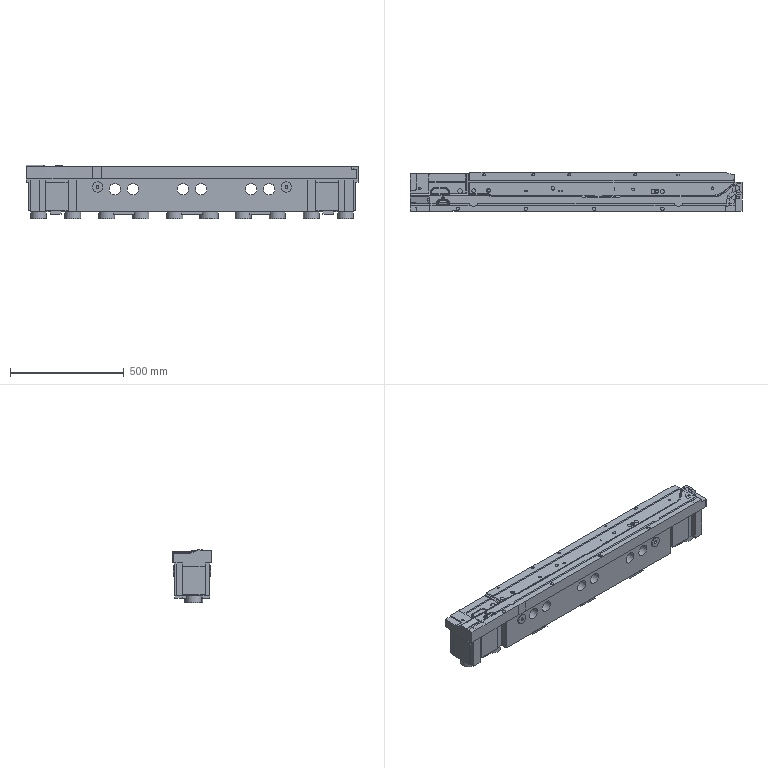Part | NX | features solid 2 | 1 solid | 330 faces | box 1460 x 171.859 x 235.617 mm | volume 41885749 mm3 | plane 145 | spline 115 | cylinder 62 | cone 6 | torus 1 | sphere 1 | commonest cylinder face diameters 12 x28 70 x9 50 x6 10 x4 40 x4 45 x4